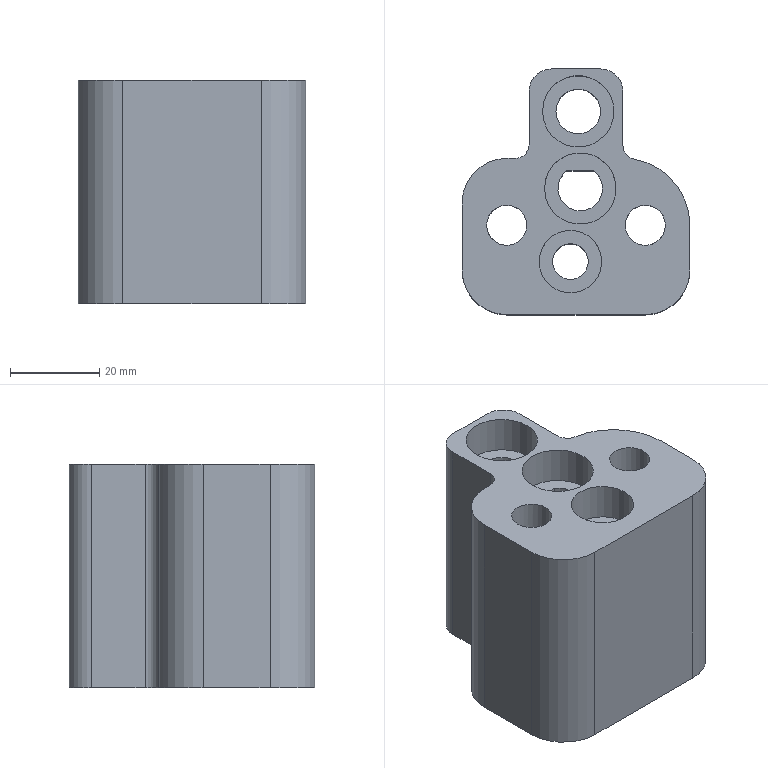Part | STEP file | PN_0021_id1034_x_t | 1 solid | 33 faces | box 51 x 55 x 50 mm | volume 79399 mm3 | cylinder 18 | plane 15 | commonest cylinder face diameters 10 x4 14 x3 20 x3 6 x2 9 x2 16 x2
STEP:
#1=CARTESIAN_POINT('',(276.,-8.,45.));
#2=VERTEX_POINT('',#1);
#3=CARTESIAN_POINT('',(276.,-20.224,45.));
#4=VERTEX_POINT('',#3);
#5=CARTESIAN_POINT('',(276.,-28.807,45.));
#6=DIRECTION('',(0.,-1.,0.));
#7=VECTOR('',#6,1.);
#8=LINE('',#5,#7);
#9=EDGE_CURVE('',#2,#4,#8,.T.);
#10=ORIENTED_EDGE('',*,*,#9,.F.);
#11=CARTESIAN_POINT('',(276.,-8.,95.));
#12=VERTEX_POINT('',#11);
#13=CARTESIAN_POINT('',(276.,-8.,95.));
#14=DIRECTION('',(0.,0.,1.));
#15=VECTOR('',#14,1.);
#16=LINE('',#13,#15);
#17=EDGE_CURVE('',#2,#12,#16,.T.);
#18=ORIENTED_EDGE('',*,*,#17,.T.);
#19=CARTESIAN_POINT('',(276.,-20.224,95.));
#20=VERTEX_POINT('',#19);
#21=CARTESIAN_POINT('',(276.,-28.807,95.));
#22=DIRECTION('',(0.,1.,0.));
#23=VECTOR('',#22,1.);
#24=LINE('',#21,#23);
#25=EDGE_CURVE('',#20,#12,#24,.T.);
#26=ORIENTED_EDGE('',*,*,#25,.F.);
#27=CARTESIAN_POINT('',(276.,-20.224,95.));
#28=DIRECTION('',(0.,0.,1.));
#29=VECTOR('',#28,1.);
#30=LINE('',#27,#29);
#31=EDGE_CURVE('',#4,#20,#30,.T.);
#32=ORIENTED_EDGE('',*,*,#31,.F.);
#33=EDGE_LOOP('',(#10,#18,#26,#32));
#34=FACE_OUTER_BOUND('',#33,.T.);
#35=CARTESIAN_POINT('',(276.,-28.807,95.));
#36=DIRECTION('',(1.,0.,0.));
#37=DIRECTION('',(0.,0.,-1.));
#38=AXIS2_PLACEMENT_3D('',#35,#36,#37);
#39=PLANE('',#38);
#40=ADVANCED_FACE('',(#34),#39,.T.);
#41=CARTESIAN_POINT('',(255.,-8.,95.));
#42=VERTEX_POINT('',#41);
#43=CARTESIAN_POINT('',(255.,-20.,95.));
#44=VERTEX_POINT('',#43);
#45=CARTESIAN_POINT('',(255.,-28.807,95.));
#46=DIRECTION('',(0.,-1.,0.));
#47=VECTOR('',#46,1.);
#48=LINE('',#45,#47);
#49=EDGE_CURVE('',#42,#44,#48,.T.);
#50=ORIENTED_EDGE('',*,*,#49,.F.);
#51=CARTESIAN_POINT('',(255.,-8.,45.));
#52=VERTEX_POINT('',#51);
#53=CARTESIAN_POINT('',(255.,-8.,95.));
#54=DIRECTION('',(0.,0.,-1.));
#55=VECTOR('',#54,1.);
#56=LINE('',#53,#55);
#57=EDGE_CURVE('',#42,#52,#56,.T.);
#58=ORIENTED_EDGE('',*,*,#57,.T.);
#59=CARTESIAN_POINT('',(255.,-20.,45.));
#60=VERTEX_POINT('',#59);
#61=CARTESIAN_POINT('',(255.,-28.807,45.));
#62=DIRECTION('',(0.,1.,0.));
#63=VECTOR('',#62,1.);
#64=LINE('',#61,#63);
#65=EDGE_CURVE('',#60,#52,#64,.T.);
#66=ORIENTED_EDGE('',*,*,#65,.F.);
#67=CARTESIAN_POINT('',(255.,-20.,95.));
#68=DIRECTION('',(0.,0.,-1.));
#69=VECTOR('',#68,1.);
#70=LINE('',#67,#69);
#71=EDGE_CURVE('',#44,#60,#70,.T.);
#72=ORIENTED_EDGE('',*,*,#71,.F.);
#73=EDGE_LOOP('',(#50,#58,#66,#72));
#74=FACE_OUTER_BOUND('',#73,.T.);
#75=CARTESIAN_POINT('',(255.,-28.807,95.));
#76=DIRECTION('',(-1.,0.,0.));
#77=DIRECTION('',(0.,0.,1.));
#78=AXIS2_PLACEMENT_3D('',#75,#76,#77);
#79=PLANE('',#78);
#80=ADVANCED_FACE('',(#74),#79,.T.);
#81=CARTESIAN_POINT('',(271.,-12.5,45.));
#82=VERTEX_POINT('',#81);
#83=CARTESIAN_POINT('',(266.,-12.5,45.));
#84=DIRECTION('',(0.,0.,-1.));
#85=DIRECTION('',(1.,0.,0.));
#86=AXIS2_PLACEMENT_3D('',#83,#84,#85);
#87=CIRCLE('',#86,5.);
#88=EDGE_CURVE('',#82,#82,#87,.T.);
#89=ORIENTED_EDGE('',*,*,#88,.F.);
#90=EDGE_LOOP('',(#89));
#91=FACE_BOUND('',#90,.T.);
#92=CARTESIAN_POINT('',(268.25,-46.114,45.));
#93=VERTEX_POINT('',#92);
#94=CARTESIAN_POINT('',(264.25,-46.114,45.));
#95=DIRECTION('',(0.,0.,-1.));
#96=DIRECTION('',(1.,0.,0.));
#97=AXIS2_PLACEMENT_3D('',#94,#95,#96);
#98=CIRCLE('',#97,4.);
#99=EDGE_CURVE('',#93,#93,#98,.T.);
#100=ORIENTED_EDGE('',*,*,#99,.F.);
#101=EDGE_LOOP('',(#100));
#102=FACE_BOUND('',#101,.T.);
#103=CARTESIAN_POINT('',(263.45,-25.762,45.));
#104=VERTEX_POINT('',#103);
#105=CARTESIAN_POINT('',(269.45,-25.762,45.));
#106=VERTEX_POINT('',#105);
#107=CARTESIAN_POINT('',(266.45,-25.762,45.));
#108=DIRECTION('',(1.,0.,0.));
#109=VECTOR('',#108,1.);
#110=LINE('',#107,#109);
#111=EDGE_CURVE('',#104,#106,#110,.T.);
#112=ORIENTED_EDGE('',*,*,#111,.F.);
#113=CARTESIAN_POINT('',(266.45,-29.762,45.));
#114=DIRECTION('',(0.,0.,-1.));
#115=DIRECTION('',(1.,0.,0.));
#116=AXIS2_PLACEMENT_3D('',#113,#114,#115);
#117=CIRCLE('',#116,5.);
#118=EDGE_CURVE('',#106,#104,#117,.T.);
#119=ORIENTED_EDGE('',*,*,#118,.F.);
#120=EDGE_LOOP('',(#112,#119));
#121=FACE_BOUND('',#120,.T.);
#122=CARTESIAN_POINT('',(250.,-31.,45.));
#123=VERTEX_POINT('',#122);
#124=CARTESIAN_POINT('',(250.,-38.,45.));
#125=DIRECTION('',(0.,0.,-1.));
#126=DIRECTION('',(0.,1.,0.));
#127=AXIS2_PLACEMENT_3D('',#124,#125,#126);
#128=CIRCLE('',#127,7.);
#129=EDGE_CURVE('',#123,#123,#128,.T.);
#130=ORIENTED_EDGE('',*,*,#129,.F.);
#131=EDGE_LOOP('',(#130));
#132=FACE_BOUND('',#131,.T.);
#133=CARTESIAN_POINT('',(281.,-45.,45.));
#134=VERTEX_POINT('',#133);
#135=CARTESIAN_POINT('',(281.,-38.,45.));
#136=DIRECTION('',(0.,0.,-1.));
#137=DIRECTION('',(0.,-1.,0.));
#138=AXIS2_PLACEMENT_3D('',#135,#136,#137);
#139=CIRCLE('',#138,7.);
#140=EDGE_CURVE('',#134,#134,#139,.T.);
#141=ORIENTED_EDGE('',*,*,#140,.F.);
#142=EDGE_LOOP('',(#141));
#143=FACE_BOUND('',#142,.T.);
#144=CARTESIAN_POINT('',(278.5,-23.182,45.));
#145=VERTEX_POINT('',#144);
#146=CARTESIAN_POINT('',(279.,-20.224,45.));
#147=DIRECTION('',(0.,0.,-1.));
#148=DIRECTION('',(1.,0.,0.));
#149=AXIS2_PLACEMENT_3D('',#146,#147,#148);
#150=CIRCLE('',#149,3.);
#151=EDGE_CURVE('',#145,#4,#150,.T.);
#152=ORIENTED_EDGE('',*,*,#151,.F.);
#153=CARTESIAN_POINT('',(291.,-37.972,45.));
#154=VERTEX_POINT('',#153);
#155=CARTESIAN_POINT('',(276.,-37.972,45.));
#156=DIRECTION('',(0.,0.,-1.));
#157=DIRECTION('',(1.,0.,0.));
#158=AXIS2_PLACEMENT_3D('',#155,#156,#157);
#159=CIRCLE('',#158,15.);
#160=EDGE_CURVE('',#145,#154,#159,.T.);
#161=ORIENTED_EDGE('',*,*,#160,.T.);
#162=CARTESIAN_POINT('',(291.,-48.,45.));
#163=VERTEX_POINT('',#162);
#164=CARTESIAN_POINT('',(291.,-28.807,45.));
#165=DIRECTION('',(0.,1.,0.));
#166=VECTOR('',#165,1.);
#167=LINE('',#164,#166);
#168=EDGE_CURVE('',#163,#154,#167,.T.);
#169=ORIENTED_EDGE('',*,*,#168,.F.);
#170=CARTESIAN_POINT('',(281.,-58.,45.));
#171=VERTEX_POINT('',#170);
#172=CARTESIAN_POINT('',(281.,-48.,45.));
#173=DIRECTION('',(0.,0.,-1.));
#174=DIRECTION('',(1.,0.,0.));
#175=AXIS2_PLACEMENT_3D('',#172,#173,#174);
#176=CIRCLE('',#175,10.);
#177=EDGE_CURVE('',#163,#171,#176,.T.);
#178=ORIENTED_EDGE('',*,*,#177,.T.);
#179=CARTESIAN_POINT('',(250.,-58.,45.));
#180=VERTEX_POINT('',#179);
#181=CARTESIAN_POINT('',(265.85,-58.,45.));
#182=DIRECTION('',(-1.,0.,0.));
#183=VECTOR('',#182,1.);
#184=LINE('',#181,#183);
#185=EDGE_CURVE('',#171,#180,#184,.T.);
#186=ORIENTED_EDGE('',*,*,#185,.T.);
#187=CARTESIAN_POINT('',(240.,-48.,45.));
#188=VERTEX_POINT('',#187);
#189=CARTESIAN_POINT('',(250.,-48.,45.));
#190=DIRECTION('',(0.,0.,-1.));
#191=DIRECTION('',(1.,0.,0.));
#192=AXIS2_PLACEMENT_3D('',#189,#190,#191);
#193=CIRCLE('',#192,10.);
#194=EDGE_CURVE('',#180,#188,#193,.T.);
#195=ORIENTED_EDGE('',*,*,#194,.T.);
#196=CARTESIAN_POINT('',(240.,-33.,45.));
#197=VERTEX_POINT('',#196);
#198=CARTESIAN_POINT('',(240.,-58.,45.));
#199=DIRECTION('',(0.,1.,0.));
#200=VECTOR('',#199,1.);
#201=LINE('',#198,#200);
#202=EDGE_CURVE('',#188,#197,#201,.T.);
#203=ORIENTED_EDGE('',*,*,#202,.T.);
#204=CARTESIAN_POINT('',(250.,-23.,45.));
#205=VERTEX_POINT('',#204);
#206=CARTESIAN_POINT('',(250.,-33.,45.));
#207=DIRECTION('',(0.,0.,-1.));
#208=DIRECTION('',(1.,0.,0.));
#209=AXIS2_PLACEMENT_3D('',#206,#207,#208);
#210=CIRCLE('',#209,10.);
#211=EDGE_CURVE('',#197,#205,#210,.T.);
#212=ORIENTED_EDGE('',*,*,#211,.T.);
#213=CARTESIAN_POINT('',(252.,-23.,45.));
#214=VERTEX_POINT('',#213);
#215=CARTESIAN_POINT('',(267.85,-23.,45.));
#216=DIRECTION('',(-1.,0.,0.));
#217=VECTOR('',#216,1.);
#218=LINE('',#215,#217);
#219=EDGE_CURVE('',#214,#205,#218,.T.);
#220=ORIENTED_EDGE('',*,*,#219,.F.);
#221=CARTESIAN_POINT('',(252.,-20.,45.));
#222=DIRECTION('',(0.,0.,-1.));
#223=DIRECTION('',(1.,0.,0.));
#224=AXIS2_PLACEMENT_3D('',#221,#222,#223);
#225=CIRCLE('',#224,3.);
#226=EDGE_CURVE('',#60,#214,#225,.T.);
#227=ORIENTED_EDGE('',*,*,#226,.F.);
#228=ORIENTED_EDGE('',*,*,#65,.T.);
#229=CARTESIAN_POINT('',(260.,-3.,45.));
#230=VERTEX_POINT('',#229);
#231=CARTESIAN_POINT('',(260.,-8.,45.));
#232=DIRECTION('',(0.,0.,-1.));
#233=DIRECTION('',(1.,0.,0.));
#234=AXIS2_PLACEMENT_3D('',#231,#232,#233);
#235=CIRCLE('',#234,5.);
#236=EDGE_CURVE('',#52,#230,#235,.T.);
#237=ORIENTED_EDGE('',*,*,#236,.T.);
#238=CARTESIAN_POINT('',(271.,-3.,45.));
#239=VERTEX_POINT('',#238);
#240=CARTESIAN_POINT('',(265.85,-3.,45.));
#241=DIRECTION('',(1.,0.,0.));
#242=VECTOR('',#241,1.);
#243=LINE('',#240,#242);
#244=EDGE_CURVE('',#230,#239,#243,.T.);
#245=ORIENTED_EDGE('',*,*,#244,.T.);
#246=CARTESIAN_POINT('',(271.,-8.,45.));
#247=DIRECTION('',(0.,0.,-1.));
#248=DIRECTION('',(1.,0.,0.));
#249=AXIS2_PLACEMENT_3D('',#246,#247,#248);
#250=CIRCLE('',#249,5.);
#251=EDGE_CURVE('',#239,#2,#250,.T.);
#252=ORIENTED_EDGE('',*,*,#251,.T.);
#253=ORIENTED_EDGE('',*,*,#9,.T.);
#254=EDGE_LOOP('',(#152,#161,#169,#178,#186,#195,#203,#212,#220,#227,#228,#237,#245,#252,#253));
#255=FACE_BOUND('',#254,.T.);
#256=CARTESIAN_POINT('',(265.85,-28.807,45.));
#257=DIRECTION('',(0.,0.,1.));
#258=DIRECTION('',(1.,0.,0.));
#259=AXIS2_PLACEMENT_3D('',#256,#257,#258);
#260=PLANE('',#259);
#261=ADVANCED_FACE('',(#91,#102,#121,#132,#143,#255),#260,.F.);
#262=ORIENTED_EDGE('',*,*,#244,.F.);
#263=CARTESIAN_POINT('',(260.,-3.,95.));
#264=VERTEX_POINT('',#263);
#265=CARTESIAN_POINT('',(260.,-3.,95.));
#266=DIRECTION('',(0.,0.,1.));
#267=VECTOR('',#266,1.);
#268=LINE('',#265,#267);
#269=EDGE_CURVE('',#230,#264,#268,.T.);
#270=ORIENTED_EDGE('',*,*,#269,.T.);
#271=CARTESIAN_POINT('',(271.,-3.,95.));
#272=VERTEX_POINT('',#271);
#273=CARTESIAN_POINT('',(265.85,-3.,95.));
#274=DIRECTION('',(-1.,0.,0.));
#275=VECTOR('',#274,1.);
#276=LINE('',#273,#275);
#277=EDGE_CURVE('',#272,#264,#276,.T.);
#278=ORIENTED_EDGE('',*,*,#277,.F.);
#279=CARTESIAN_POINT('',(271.,-3.,95.));
#280=DIRECTION('',(0.,0.,-1.));
#281=VECTOR('',#280,1.);
#282=LINE('',#279,#281);
#283=EDGE_CURVE('',#272,#239,#282,.T.);
#284=ORIENTED_EDGE('',*,*,#283,.T.);
#285=EDGE_LOOP('',(#262,#270,#278,#284));
#286=FACE_OUTER_BOUND('',#285,.T.);
#287=CARTESIAN_POINT('',(265.85,-3.,95.));
#288=DIRECTION('',(0.,1.,0.));
#289=DIRECTION('',(0.,0.,-1.));
#290=AXIS2_PLACEMENT_3D('',#287,#288,#289);
#291=PLANE('',#290);
#292=ADVANCED_FACE('',(#286),#291,.T.);
#293=ORIENTED_EDGE('',*,*,#185,.F.);
#294=CARTESIAN_POINT('',(281.,-58.,95.));
#295=VERTEX_POINT('',#294);
#296=CARTESIAN_POINT('',(281.,-58.,95.));
#297=DIRECTION('',(0.,0.,1.));
#298=VECTOR('',#297,1.);
#299=LINE('',#296,#298);
#300=EDGE_CURVE('',#171,#295,#299,.T.);
#301=ORIENTED_EDGE('',*,*,#300,.T.);
#302=CARTESIAN_POINT('',(250.,-58.,95.));
#303=VERTEX_POINT('',#302);
#304=CARTESIAN_POINT('',(265.85,-58.,95.));
#305=DIRECTION('',(1.,0.,0.));
#306=VECTOR('',#305,1.);
#307=LINE('',#304,#306);
#308=EDGE_CURVE('',#303,#295,#307,.T.);
#309=ORIENTED_EDGE('',*,*,#308,.F.);
#310=CARTESIAN_POINT('',(250.,-58.,45.));
#311=DIRECTION('',(0.,0.,-1.));
#312=VECTOR('',#311,1.);
#313=LINE('',#310,#312);
#314=EDGE_CURVE('',#303,#180,#313,.T.);
#315=ORIENTED_EDGE('',*,*,#314,.T.);
#316=EDGE_LOOP('',(#293,#301,#309,#315));
#317=FACE_OUTER_BOUND('',#316,.T.);
#318=CARTESIAN_POINT('',(265.85,-58.,95.));
#319=DIRECTION('',(0.,-1.,0.));
#320=DIRECTION('',(0.,0.,1.));
#321=AXIS2_PLACEMENT_3D('',#318,#319,#320);
#322=PLANE('',#321);
#323=ADVANCED_FACE('',(#317),#322,.T.);
#324=CARTESIAN_POINT('',(274.,-12.5,95.));
#325=VERTEX_POINT('',#324);
#326=CARTESIAN_POINT('',(266.,-12.5,95.));
#327=DIRECTION('',(0.,0.,1.));
#328=DIRECTION('',(1.,0.,0.));
#329=AXIS2_PLACEMENT_3D('',#326,#327,#328);
#330=CIRCLE('',#329,8.);
#331=EDGE_CURVE('',#325,#325,#330,.T.);
#332=ORIENTED_EDGE('',*,*,#331,.F.);
#333=EDGE_LOOP('',(#332));
#334=FACE_BOUND('',#333,.T.);
#335=CARTESIAN_POINT('',(271.25,-46.114,95.));
#336=VERTEX_POINT('',#335);
#337=CARTESIAN_POINT('',(264.25,-46.114,95.));
#338=DIRECTION('',(0.,0.,1.));
#339=DIRECTION('',(1.,0.,0.));
#340=AXIS2_PLACEMENT_3D('',#337,#338,#339);
#341=CIRCLE('',#340,7.);
#342=EDGE_CURVE('',#336,#336,#341,.T.);
#343=ORIENTED_EDGE('',*,*,#342,.F.);
#344=EDGE_LOOP('',(#343));
#345=FACE_BOUND('',#344,.T.);
#346=CARTESIAN_POINT('',(274.45,-29.762,95.));
#347=VERTEX_POINT('',#346);
#348=CARTESIAN_POINT('',(266.45,-29.762,95.));
#349=DIRECTION('',(0.,0.,1.));
#350=DIRECTION('',(1.,0.,0.));
#351=AXIS2_PLACEMENT_3D('',#348,#349,#350);
#352=CIRCLE('',#351,8.);
#353=EDGE_CURVE('',#347,#347,#352,.T.);
#354=ORIENTED_EDGE('',*,*,#353,.F.);
#355=EDGE_LOOP('',(#354));
#356=FACE_BOUND('',#355,.T.);
#357=CARTESIAN_POINT('',(254.5,-38.,95.));
#358=VERTEX_POINT('',#357);
#359=CARTESIAN_POINT('',(250.,-38.,95.));
#360=DIRECTION('',(0.,0.,1.));
#361=DIRECTION('',(1.,0.,0.));
#362=AXIS2_PLACEMENT_3D('',#359,#360,#361);
#363=CIRCLE('',#362,4.5);
#364=EDGE_CURVE('',#358,#358,#363,.T.);
#365=ORIENTED_EDGE('',*,*,#364,.F.);
#366=EDGE_LOOP('',(#365));
#367=FACE_BOUND('',#366,.T.);
#368=CARTESIAN_POINT('',(285.5,-38.,95.));
#369=VERTEX_POINT('',#368);
#370=CARTESIAN_POINT('',(281.,-38.,95.));
#371=DIRECTION('',(0.,0.,1.));
#372=DIRECTION('',(1.,0.,0.));
#373=AXIS2_PLACEMENT_3D('',#370,#371,#372);
#374=CIRCLE('',#373,4.5);
#375=EDGE_CURVE('',#369,#369,#374,.T.);
#376=ORIENTED_EDGE('',*,*,#375,.F.);
#377=EDGE_LOOP('',(#376));
#378=FACE_BOUND('',#377,.T.);
#379=CARTESIAN_POINT('',(291.,-48.,95.));
#380=VERTEX_POINT('',#379);
#381=CARTESIAN_POINT('',(291.,-37.972,95.));
#382=VERTEX_POINT('',#381);
#383=CARTESIAN_POINT('',(291.,-58.,95.));
#384=DIRECTION('',(0.,1.,0.));
#385=VECTOR('',#384,1.);
#386=LINE('',#383,#385);
#387=EDGE_CURVE('',#380,#382,#386,.T.);
#388=ORIENTED_EDGE('',*,*,#387,.T.);
#389=CARTESIAN_POINT('',(278.5,-23.182,95.));
#390=VERTEX_POINT('',#389);
#391=CARTESIAN_POINT('',(276.,-37.972,95.));
#392=DIRECTION('',(0.,0.,1.));
#393=DIRECTION('',(1.,0.,0.));
#394=AXIS2_PLACEMENT_3D('',#391,#392,#393);
#395=CIRCLE('',#394,15.);
#396=EDGE_CURVE('',#382,#390,#395,.T.);
#397=ORIENTED_EDGE('',*,*,#396,.T.);
#398=CARTESIAN_POINT('',(279.,-20.224,95.));
#399=DIRECTION('',(0.,0.,1.));
#400=DIRECTION('',(1.,0.,0.));
#401=AXIS2_PLACEMENT_3D('',#398,#399,#400);
#402=CIRCLE('',#401,3.);
#403=EDGE_CURVE('',#20,#390,#402,.T.);
#404=ORIENTED_EDGE('',*,*,#403,.F.);
#405=ORIENTED_EDGE('',*,*,#25,.T.);
#406=CARTESIAN_POINT('',(271.,-8.,95.));
#407=DIRECTION('',(0.,0.,1.));
#408=DIRECTION('',(1.,0.,0.));
#409=AXIS2_PLACEMENT_3D('',#406,#407,#408);
#410=CIRCLE('',#409,5.);
#411=EDGE_CURVE('',#12,#272,#410,.T.);
#412=ORIENTED_EDGE('',*,*,#411,.T.);
#413=ORIENTED_EDGE('',*,*,#277,.T.);
#414=CARTESIAN_POINT('',(260.,-8.,95.));
#415=DIRECTION('',(0.,0.,1.));
#416=DIRECTION('',(1.,0.,0.));
#417=AXIS2_PLACEMENT_3D('',#414,#415,#416);
#418=CIRCLE('',#417,5.);
#419=EDGE_CURVE('',#264,#42,#418,.T.);
#420=ORIENTED_EDGE('',*,*,#419,.T.);
#421=ORIENTED_EDGE('',*,*,#49,.T.);
#422=CARTESIAN_POINT('',(252.,-23.,95.));
#423=VERTEX_POINT('',#422);
#424=CARTESIAN_POINT('',(252.,-20.,95.));
#425=DIRECTION('',(0.,0.,1.));
#426=DIRECTION('',(1.,0.,0.));
#427=AXIS2_PLACEMENT_3D('',#424,#425,#426);
#428=CIRCLE('',#427,3.);
#429=EDGE_CURVE('',#423,#44,#428,.T.);
#430=ORIENTED_EDGE('',*,*,#429,.F.);
#431=CARTESIAN_POINT('',(250.,-23.,95.));
#432=VERTEX_POINT('',#431);
#433=CARTESIAN_POINT('',(267.85,-23.,95.));
#434=DIRECTION('',(1.,0.,0.));
#435=VECTOR('',#434,1.);
#436=LINE('',#433,#435);
#437=EDGE_CURVE('',#432,#423,#436,.T.);
#438=ORIENTED_EDGE('',*,*,#437,.F.);
#439=CARTESIAN_POINT('',(240.,-33.,95.));
#440=VERTEX_POINT('',#439);
#441=CARTESIAN_POINT('',(250.,-33.,95.));
#442=DIRECTION('',(0.,0.,1.));
#443=DIRECTION('',(1.,0.,0.));
#444=AXIS2_PLACEMENT_3D('',#441,#442,#443);
#445=CIRCLE('',#444,10.);
#446=EDGE_CURVE('',#432,#440,#445,.T.);
#447=ORIENTED_EDGE('',*,*,#446,.T.);
#448=CARTESIAN_POINT('',(240.,-48.,95.));
#449=VERTEX_POINT('',#448);
#450=CARTESIAN_POINT('',(240.,-28.807,95.));
#451=DIRECTION('',(0.,1.,0.));
#452=VECTOR('',#451,1.);
#453=LINE('',#450,#452);
#454=EDGE_CURVE('',#449,#440,#453,.T.);
#455=ORIENTED_EDGE('',*,*,#454,.F.);
#456=CARTESIAN_POINT('',(250.,-48.,95.));
#457=DIRECTION('',(0.,0.,1.));
#458=DIRECTION('',(1.,0.,0.));
#459=AXIS2_PLACEMENT_3D('',#456,#457,#458);
#460=CIRCLE('',#459,10.);
#461=EDGE_CURVE('',#449,#303,#460,.T.);
#462=ORIENTED_EDGE('',*,*,#461,.T.);
#463=ORIENTED_EDGE('',*,*,#308,.T.);
#464=CARTESIAN_POINT('',(281.,-48.,95.));
#465=DIRECTION('',(0.,0.,1.));
#466=DIRECTION('',(1.,0.,0.));
#467=AXIS2_PLACEMENT_3D('',#464,#465,#466);
#468=CIRCLE('',#467,10.);
#469=EDGE_CURVE('',#295,#380,#468,.T.);
#470=ORIENTED_EDGE('',*,*,#469,.T.);
#471=EDGE_LOOP('',(#388,#397,#404,#405,#412,#413,#420,#421,#430,#438,#447,#455,#462,#463,#470));
#472=FACE_BOUND('',#471,.T.);
#473=CARTESIAN_POINT('',(265.85,-28.807,95.));
#474=DIRECTION('',(0.,0.,1.));
#475=DIRECTION('',(1.,0.,0.));
#476=AXIS2_PLACEMENT_3D('',#473,#474,#475);
#477=PLANE('',#476);
#478=ADVANCED_FACE('',(#334,#345,#356,#367,#378,#472),#477,.T.);
#479=ORIENTED_EDGE('',*,*,#454,.T.);
#480=CARTESIAN_POINT('',(240.,-33.,95.));
#481=DIRECTION('',(0.,0.,-1.));
#482=VECTOR('',#481,1.);
#483=LINE('',#480,#482);
#484=EDGE_CURVE('',#440,#197,#483,.T.);
#485=ORIENTED_EDGE('',*,*,#484,.T.);
#486=ORIENTED_EDGE('',*,*,#202,.F.);
#487=CARTESIAN_POINT('',(240.,-48.,95.));
#488=DIRECTION('',(0.,0.,1.));
#489=VECTOR('',#488,1.);
#490=LINE('',#487,#489);
#491=EDGE_CURVE('',#188,#449,#490,.T.);
#492=ORIENTED_EDGE('',*,*,#491,.T.);
#493=EDGE_LOOP('',(#479,#485,#486,#492));
#494=FACE_OUTER_BOUND('',#493,.T.);
#495=CARTESIAN_POINT('',(240.,-58.,95.));
#496=DIRECTION('',(1.,0.,0.));
#497=DIRECTION('',(0.,0.,-1.));
#498=AXIS2_PLACEMENT_3D('',#495,#496,#497);
#499=PLANE('',#498);
#500=ADVANCED_FACE('',(#494),#499,.F.);
#501=ORIENTED_EDGE('',*,*,#219,.T.);
#502=CARTESIAN_POINT('',(250.,-23.,95.));
#503=DIRECTION('',(0.,0.,1.));
#504=VECTOR('',#503,1.);
#505=LINE('',#502,#504);
#506=EDGE_CURVE('',#205,#432,#505,.T.);
#507=ORIENTED_EDGE('',*,*,#506,.T.);
#508=ORIENTED_EDGE('',*,*,#437,.T.);
#509=CARTESIAN_POINT('',(252.,-23.,95.));
#510=DIRECTION('',(0.,0.,1.));
#511=VECTOR('',#510,1.);
#512=LINE('',#509,#511);
#513=EDGE_CURVE('',#214,#423,#512,.T.);
#514=ORIENTED_EDGE('',*,*,#513,.F.);
#515=EDGE_LOOP('',(#501,#507,#508,#514));
#516=FACE_OUTER_BOUND('',#515,.T.);
#517=CARTESIAN_POINT('',(267.85,-23.,95.));
#518=DIRECTION('',(0.,-1.,0.));
#519=DIRECTION('',(0.,0.,1.));
#520=AXIS2_PLACEMENT_3D('',#517,#518,#519);
#521=PLANE('',#520);
#522=ADVANCED_FACE('',(#516),#521,.F.);
#523=ORIENTED_EDGE('',*,*,#168,.T.);
#524=CARTESIAN_POINT('',(291.,-37.972,95.));
#525=DIRECTION('',(0.,0.,1.));
#526=VECTOR('',#525,1.);
#527=LINE('',#524,#526);
#528=EDGE_CURVE('',#154,#382,#527,.T.);
#529=ORIENTED_EDGE('',*,*,#528,.T.);
#530=ORIENTED_EDGE('',*,*,#387,.F.);
#531=CARTESIAN_POINT('',(291.,-48.,45.));
#532=DIRECTION('',(0.,0.,-1.));
#533=VECTOR('',#532,1.);
#534=LINE('',#531,#533);
#535=EDGE_CURVE('',#380,#163,#534,.T.);
#536=ORIENTED_EDGE('',*,*,#535,.T.);
#537=EDGE_LOOP('',(#523,#529,#530,#536));
#538=FACE_OUTER_BOUND('',#537,.T.);
#539=CARTESIAN_POINT('',(291.,-58.,95.));
#540=DIRECTION('',(1.,0.,0.));
#541=DIRECTION('',(0.,0.,-1.));
#542=AXIS2_PLACEMENT_3D('',#539,#540,#541);
#543=PLANE('',#542);
#544=ADVANCED_FACE('',(#538),#543,.T.);
#545=ORIENTED_EDGE('',*,*,#403,.T.);
#546=CARTESIAN_POINT('',(278.5,-23.182,95.));
#547=DIRECTION('',(0.,0.,-1.));
#548=VECTOR('',#547,1.);
#549=LINE('',#546,#548);
#550=EDGE_CURVE('',#390,#145,#549,.T.);
#551=ORIENTED_EDGE('',*,*,#550,.T.);
#552=ORIENTED_EDGE('',*,*,#151,.T.);
#553=ORIENTED_EDGE('',*,*,#31,.T.);
#554=EDGE_LOOP('',(#545,#551,#552,#553));
#555=FACE_OUTER_BOUND('',#554,.T.);
#556=CARTESIAN_POINT('',(279.,-20.224,95.));
#557=DIRECTION('',(0.,0.,1.));
#558=DIRECTION('',(1.,0.,0.));
#559=AXIS2_PLACEMENT_3D('',#556,#557,#558);
#560=CYLINDRICAL_SURFACE('',#559,3.);
#561=ADVANCED_FACE('',(#555),#560,.F.);
#562=ORIENTED_EDGE('',*,*,#429,.T.);
#563=ORIENTED_EDGE('',*,*,#71,.T.);
#564=ORIENTED_EDGE('',*,*,#226,.T.);
#565=ORIENTED_EDGE('',*,*,#513,.T.);
#566=EDGE_LOOP('',(#562,#563,#564,#565));
#567=FACE_OUTER_BOUND('',#566,.T.);
#568=CARTESIAN_POINT('',(252.,-20.,95.));
#569=DIRECTION('',(0.,0.,-1.));
#570=DIRECTION('',(-1.,0.,0.));
#571=AXIS2_PLACEMENT_3D('',#568,#569,#570);
#572=CYLINDRICAL_SURFACE('',#571,3.);
#573=ADVANCED_FACE('',(#567),#572,.F.);
#574=ORIENTED_EDGE('',*,*,#446,.F.);
#575=ORIENTED_EDGE('',*,*,#506,.F.);
#576=ORIENTED_EDGE('',*,*,#211,.F.);
#577=ORIENTED_EDGE('',*,*,#484,.F.);
#578=EDGE_LOOP('',(#574,#575,#576,#577));
#579=FACE_OUTER_BOUND('',#578,.T.);
#580=CARTESIAN_POINT('',(250.,-33.,95.));
#581=DIRECTION('',(0.,0.,-1.));
#582=DIRECTION('',(-1.,0.,0.));
#583=AXIS2_PLACEMENT_3D('',#580,#581,#582);
#584=CYLINDRICAL_SURFACE('',#583,10.);
#585=ADVANCED_FACE('',(#579),#584,.T.);
#586=ORIENTED_EDGE('',*,*,#469,.F.);
#587=ORIENTED_EDGE('',*,*,#300,.F.);
#588=ORIENTED_EDGE('',*,*,#177,.F.);
#589=ORIENTED_EDGE('',*,*,#535,.F.);
#590=EDGE_LOOP('',(#586,#587,#588,#589));
#591=FACE_OUTER_BOUND('',#590,.T.);
#592=CARTESIAN_POINT('',(281.,-48.,95.));
#593=DIRECTION('',(0.,0.,-1.));
#594=DIRECTION('',(-1.,0.,0.));
#595=AXIS2_PLACEMENT_3D('',#592,#593,#594);
#596=CYLINDRICAL_SURFACE('',#595,10.);
#597=ADVANCED_FACE('',(#591),#596,.T.);
#598=ORIENTED_EDGE('',*,*,#461,.F.);
#599=ORIENTED_EDGE('',*,*,#491,.F.);
#600=ORIENTED_EDGE('',*,*,#194,.F.);
#601=ORIENTED_EDGE('',*,*,#314,.F.);
#602=EDGE_LOOP('',(#598,#599,#600,#601));
#603=FACE_OUTER_BOUND('',#602,.T.);
#604=CARTESIAN_POINT('',(250.,-48.,95.));
#605=DIRECTION('',(0.,0.,1.));
#606=DIRECTION('',(1.,0.,0.));
#607=AXIS2_PLACEMENT_3D('',#604,#605,#606);
#608=CYLINDRICAL_SURFACE('',#607,10.);
#609=ADVANCED_FACE('',(#603),#608,.T.);
#610=ORIENTED_EDGE('',*,*,#419,.F.);
#611=ORIENTED_EDGE('',*,*,#269,.F.);
#612=ORIENTED_EDGE('',*,*,#236,.F.);
#613=ORIENTED_EDGE('',*,*,#57,.F.);
#614=EDGE_LOOP('',(#610,#611,#612,#613));
#615=FACE_OUTER_BOUND('',#614,.T.);
#616=CARTESIAN_POINT('',(260.,-8.,95.));
#617=DIRECTION('',(0.,0.,-1.));
#618=DIRECTION('',(-1.,0.,0.));
#619=AXIS2_PLACEMENT_3D('',#616,#617,#618);
#620=CYLINDRICAL_SURFACE('',#619,5.);
#621=ADVANCED_FACE('',(#615),#620,.T.);
#622=ORIENTED_EDGE('',*,*,#411,.F.);
#623=ORIENTED_EDGE('',*,*,#17,.F.);
#624=ORIENTED_EDGE('',*,*,#251,.F.);
#625=ORIENTED_EDGE('',*,*,#283,.F.);
#626=EDGE_LOOP('',(#622,#623,#624,#625));
#627=FACE_OUTER_BOUND('',#626,.T.);
#628=CARTESIAN_POINT('',(271.,-8.,95.));
#629=DIRECTION('',(0.,0.,-1.));
#630=DIRECTION('',(-1.,0.,0.));
#631=AXIS2_PLACEMENT_3D('',#628,#629,#630);
#632=CYLINDRICAL_SURFACE('',#631,5.);
#633=ADVANCED_FACE('',(#627),#632,.T.);
#634=ORIENTED_EDGE('',*,*,#396,.F.);
#635=ORIENTED_EDGE('',*,*,#528,.F.);
#636=ORIENTED_EDGE('',*,*,#160,.F.);
#637=ORIENTED_EDGE('',*,*,#550,.F.);
#638=EDGE_LOOP('',(#634,#635,#636,#637));
#639=FACE_OUTER_BOUND('',#638,.T.);
#640=CARTESIAN_POINT('',(276.,-37.972,95.));
#641=DIRECTION('',(0.,0.,1.));
#642=DIRECTION('',(1.,0.,0.));
#643=AXIS2_PLACEMENT_3D('',#640,#641,#642);
#644=CYLINDRICAL_SURFACE('',#643,15.);
#645=ADVANCED_FACE('',(#639),#644,.T.);
#646=ORIENTED_EDGE('',*,*,#375,.T.);
#647=EDGE_LOOP('',(#646));
#648=FACE_BOUND('',#647,.T.);
#649=CARTESIAN_POINT('',(281.,-42.5,75.));
#650=VERTEX_POINT('',#649);
#651=CARTESIAN_POINT('',(281.,-38.,75.));
#652=DIRECTION('',(0.,0.,-1.));
#653=DIRECTION('',(0.,-1.,0.));
#654=AXIS2_PLACEMENT_3D('',#651,#652,#653);
#655=CIRCLE('',#654,4.5);
#656=EDGE_CURVE('',#650,#650,#655,.T.);
#657=ORIENTED_EDGE('',*,*,#656,.T.);
#658=EDGE_LOOP('',(#657));
#659=FACE_BOUND('',#658,.T.);
#660=CARTESIAN_POINT('',(281.,-38.,105.));
#661=DIRECTION('',(0.,0.,-1.));
#662=DIRECTION('',(0.,1.,0.));
#663=AXIS2_PLACEMENT_3D('',#660,#661,#662);
#664=CYLINDRICAL_SURFACE('',#663,4.5);
#665=ADVANCED_FACE('',(#648,#659),#664,.F.);
#666=ORIENTED_EDGE('',*,*,#656,.F.);
#667=EDGE_LOOP('',(#666));
#668=FACE_BOUND('',#667,.T.);
#669=CARTESIAN_POINT('',(281.,-31.,75.));
#670=VERTEX_POINT('',#669);
#671=CARTESIAN_POINT('',(281.,-38.,75.));
#672=DIRECTION('',(0.,0.,-1.));
#673=DIRECTION('',(0.,1.,0.));
#674=AXIS2_PLACEMENT_3D('',#671,#672,#673);
#675=CIRCLE('',#674,7.);
#676=EDGE_CURVE('',#670,#670,#675,.T.);
#677=ORIENTED_EDGE('',*,*,#676,.T.);
#678=EDGE_LOOP('',(#677));
#679=FACE_BOUND('',#678,.T.);
#680=CARTESIAN_POINT('',(281.,-38.,75.));
#681=DIRECTION('',(0.,0.,1.));
#682=DIRECTION('',(0.,-1.,0.));
#683=AXIS2_PLACEMENT_3D('',#680,#681,#682);
#684=PLANE('',#683);
#685=ADVANCED_FACE('',(#668,#679),#684,.F.);
#686=ORIENTED_EDGE('',*,*,#140,.T.);
#687=EDGE_LOOP('',(#686));
#688=FACE_BOUND('',#687,.T.);
#689=ORIENTED_EDGE('',*,*,#676,.F.);
#690=EDGE_LOOP('',(#689));
#691=FACE_BOUND('',#690,.T.);
#692=CARTESIAN_POINT('',(281.,-38.,75.));
#693=DIRECTION('',(0.,0.,-1.));
#694=DIRECTION('',(0.,1.,0.));
#695=AXIS2_PLACEMENT_3D('',#692,#693,#694);
#696=CYLINDRICAL_SURFACE('',#695,7.);
#697=ADVANCED_FACE('',(#688,#691),#696,.F.);
#698=ORIENTED_EDGE('',*,*,#364,.T.);
#699=EDGE_LOOP('',(#698));
#700=FACE_BOUND('',#699,.T.);
#701=CARTESIAN_POINT('',(250.,-33.5,75.));
#702=VERTEX_POINT('',#701);
#703=CARTESIAN_POINT('',(250.,-38.,75.));
#704=DIRECTION('',(0.,0.,-1.));
#705=DIRECTION('',(0.,1.,0.));
#706=AXIS2_PLACEMENT_3D('',#703,#704,#705);
#707=CIRCLE('',#706,4.5);
#708=EDGE_CURVE('',#702,#702,#707,.T.);
#709=ORIENTED_EDGE('',*,*,#708,.T.);
#710=EDGE_LOOP('',(#709));
#711=FACE_BOUND('',#710,.T.);
#712=CARTESIAN_POINT('',(250.,-38.,105.));
#713=DIRECTION('',(0.,0.,-1.));
#714=DIRECTION('',(0.,-1.,0.));
#715=AXIS2_PLACEMENT_3D('',#712,#713,#714);
#716=CYLINDRICAL_SURFACE('',#715,4.5);
#717=ADVANCED_FACE('',(#700,#711),#716,.F.);
#718=ORIENTED_EDGE('',*,*,#708,.F.);
#719=EDGE_LOOP('',(#718));
#720=FACE_BOUND('',#719,.T.);
#721=CARTESIAN_POINT('',(250.,-45.,75.));
#722=VERTEX_POINT('',#721);
#723=CARTESIAN_POINT('',(250.,-38.,75.));
#724=DIRECTION('',(0.,0.,-1.));
#725=DIRECTION('',(0.,-1.,0.));
#726=AXIS2_PLACEMENT_3D('',#723,#724,#725);
#727=CIRCLE('',#726,7.);
#728=EDGE_CURVE('',#722,#722,#727,.T.);
#729=ORIENTED_EDGE('',*,*,#728,.T.);
#730=EDGE_LOOP('',(#729));
#731=FACE_BOUND('',#730,.T.);
#732=CARTESIAN_POINT('',(250.,-38.,75.));
#733=DIRECTION('',(0.,0.,1.));
#734=DIRECTION('',(0.,1.,0.));
#735=AXIS2_PLACEMENT_3D('',#732,#733,#734);
#736=PLANE('',#735);
#737=ADVANCED_FACE('',(#720,#731),#736,.F.);
#738=ORIENTED_EDGE('',*,*,#129,.T.);
#739=EDGE_LOOP('',(#738));
#740=FACE_BOUND('',#739,.T.);
#741=ORIENTED_EDGE('',*,*,#728,.F.);
#742=EDGE_LOOP('',(#741));
#743=FACE_BOUND('',#742,.T.);
#744=CARTESIAN_POINT('',(250.,-38.,75.));
#745=DIRECTION('',(0.,0.,-1.));
#746=DIRECTION('',(0.,-1.,0.));
#747=AXIS2_PLACEMENT_3D('',#744,#745,#746);
#748=CYLINDRICAL_SURFACE('',#747,7.);
#749=ADVANCED_FACE('',(#740,#743),#748,.F.);
#750=CARTESIAN_POINT('',(269.45,-25.762,86.7));
#751=VERTEX_POINT('',#750);
#752=CARTESIAN_POINT('',(263.45,-25.762,86.7));
#753=VERTEX_POINT('',#752);
#754=CARTESIAN_POINT('',(266.45,-25.762,86.7));
#755=DIRECTION('',(-1.,0.,0.));
#756=VECTOR('',#755,1.);
#757=LINE('',#754,#756);
#758=EDGE_CURVE('',#751,#753,#757,.T.);
#759=ORIENTED_EDGE('',*,*,#758,.F.);
#760=CARTESIAN_POINT('',(266.45,-29.762,86.7));
#761=DIRECTION('',(0.,0.,-1.));
#762=DIRECTION('',(-1.,0.,0.));
#763=AXIS2_PLACEMENT_3D('',#760,#761,#762);
#764=CIRCLE('',#763,5.);
#765=EDGE_CURVE('',#751,#753,#764,.T.);
#766=ORIENTED_EDGE('',*,*,#765,.T.);
#767=EDGE_LOOP('',(#759,#766));
#768=FACE_BOUND('',#767,.T.);
#769=CARTESIAN_POINT('',(258.45,-29.762,86.7));
#770=VERTEX_POINT('',#769);
#771=CARTESIAN_POINT('',(266.45,-29.762,86.7));
#772=DIRECTION('',(0.,0.,1.));
#773=DIRECTION('',(-1.,0.,0.));
#774=AXIS2_PLACEMENT_3D('',#771,#772,#773);
#775=CIRCLE('',#774,8.);
#776=EDGE_CURVE('',#770,#770,#775,.T.);
#777=ORIENTED_EDGE('',*,*,#776,.T.);
#778=EDGE_LOOP('',(#777));
#779=FACE_BOUND('',#778,.T.);
#780=CARTESIAN_POINT('',(266.45,-29.762,86.7));
#781=DIRECTION('',(0.,0.,-1.));
#782=DIRECTION('',(-1.,0.,0.));
#783=AXIS2_PLACEMENT_3D('',#780,#781,#782);
#784=PLANE('',#783);
#785=ADVANCED_FACE('',(#768,#779),#784,.F.);
#786=ORIENTED_EDGE('',*,*,#776,.F.);
#787=EDGE_LOOP('',(#786));
#788=FACE_BOUND('',#787,.T.);
#789=ORIENTED_EDGE('',*,*,#353,.T.);
#790=EDGE_LOOP('',(#789));
#791=FACE_BOUND('',#790,.T.);
#792=CARTESIAN_POINT('',(266.45,-29.762,94.559));
#793=DIRECTION('',(0.,0.,-1.));
#794=DIRECTION('',(0.,1.,0.));
#795=AXIS2_PLACEMENT_3D('',#792,#793,#794);
#796=CYLINDRICAL_SURFACE('',#795,8.);
#797=ADVANCED_FACE('',(#788,#791),#796,.F.);
#798=CARTESIAN_POINT('',(269.45,-25.762,85.5));
#799=DIRECTION('',(0.,0.,1.));
#800=VECTOR('',#799,1.);
#801=LINE('',#798,#800);
#802=EDGE_CURVE('',#106,#751,#801,.T.);
#803=ORIENTED_EDGE('',*,*,#802,.T.);
#804=ORIENTED_EDGE('',*,*,#758,.T.);
#805=CARTESIAN_POINT('',(263.45,-25.762,85.5));
#806=DIRECTION('',(0.,0.,-1.));
#807=VECTOR('',#806,1.);
#808=LINE('',#805,#807);
#809=EDGE_CURVE('',#753,#104,#808,.T.);
#810=ORIENTED_EDGE('',*,*,#809,.T.);
#811=ORIENTED_EDGE('',*,*,#111,.T.);
#812=EDGE_LOOP('',(#803,#804,#810,#811));
#813=FACE_OUTER_BOUND('',#812,.T.);
#814=CARTESIAN_POINT('',(266.45,-25.762,56.595));
#815=DIRECTION('',(0.,1.,0.));
#816=DIRECTION('',(0.,0.,-1.));
#817=AXIS2_PLACEMENT_3D('',#814,#815,#816);
#818=PLANE('',#817);
#819=ADVANCED_FACE('',(#813),#818,.F.);
#820=ORIENTED_EDGE('',*,*,#118,.T.);
#821=ORIENTED_EDGE('',*,*,#809,.F.);
#822=ORIENTED_EDGE('',*,*,#765,.F.);
#823=ORIENTED_EDGE('',*,*,#802,.F.);
#824=EDGE_LOOP('',(#820,#821,#822,#823));
#825=FACE_OUTER_BOUND('',#824,.T.);
#826=CARTESIAN_POINT('',(266.45,-29.762,85.5));
#827=DIRECTION('',(0.,0.,-1.));
#828=DIRECTION('',(0.,1.,0.));
#829=AXIS2_PLACEMENT_3D('',#826,#827,#828);
#830=CYLINDRICAL_SURFACE('',#829,5.);
#831=ADVANCED_FACE('',(#825),#830,.F.);
#832=CARTESIAN_POINT('',(260.25,-46.114,86.7));
#833=VERTEX_POINT('',#832);
#834=CARTESIAN_POINT('',(264.25,-46.114,86.7));
#835=DIRECTION('',(0.,0.,-1.));
#836=DIRECTION('',(-1.,0.,0.));
#837=AXIS2_PLACEMENT_3D('',#834,#835,#836);
#838=CIRCLE('',#837,4.);
#839=EDGE_CURVE('',#833,#833,#838,.T.);
#840=ORIENTED_EDGE('',*,*,#839,.T.);
#841=EDGE_LOOP('',(#840));
#842=FACE_BOUND('',#841,.T.);
#843=CARTESIAN_POINT('',(257.25,-46.114,86.7));
#844=VERTEX_POINT('',#843);
#845=CARTESIAN_POINT('',(264.25,-46.114,86.7));
#846=DIRECTION('',(0.,0.,1.));
#847=DIRECTION('',(-1.,0.,0.));
#848=AXIS2_PLACEMENT_3D('',#845,#846,#847);
#849=CIRCLE('',#848,7.);
#850=EDGE_CURVE('',#844,#844,#849,.T.);
#851=ORIENTED_EDGE('',*,*,#850,.T.);
#852=EDGE_LOOP('',(#851));
#853=FACE_BOUND('',#852,.T.);
#854=CARTESIAN_POINT('',(264.25,-46.114,86.7));
#855=DIRECTION('',(0.,0.,-1.));
#856=DIRECTION('',(-1.,0.,0.));
#857=AXIS2_PLACEMENT_3D('',#854,#855,#856);
#858=PLANE('',#857);
#859=ADVANCED_FACE('',(#842,#853),#858,.F.);
#860=ORIENTED_EDGE('',*,*,#850,.F.);
#861=EDGE_LOOP('',(#860));
#862=FACE_BOUND('',#861,.T.);
#863=ORIENTED_EDGE('',*,*,#342,.T.);
#864=EDGE_LOOP('',(#863));
#865=FACE_BOUND('',#864,.T.);
#866=CARTESIAN_POINT('',(264.25,-46.114,94.559));
#867=DIRECTION('',(0.,0.,-1.));
#868=DIRECTION('',(0.,1.,0.));
#869=AXIS2_PLACEMENT_3D('',#866,#867,#868);
#870=CYLINDRICAL_SURFACE('',#869,7.);
#871=ADVANCED_FACE('',(#862,#865),#870,.F.);
#872=ORIENTED_EDGE('',*,*,#839,.F.);
#873=EDGE_LOOP('',(#872));
#874=FACE_BOUND('',#873,.T.);
#875=ORIENTED_EDGE('',*,*,#99,.T.);
#876=EDGE_LOOP('',(#875));
#877=FACE_BOUND('',#876,.T.);
#878=CARTESIAN_POINT('',(264.25,-46.114,85.5));
#879=DIRECTION('',(0.,0.,-1.));
#880=DIRECTION('',(0.,1.,0.));
#881=AXIS2_PLACEMENT_3D('',#878,#879,#880);
#882=CYLINDRICAL_SURFACE('',#881,4.);
#883=ADVANCED_FACE('',(#874,#877),#882,.F.);
#884=CARTESIAN_POINT('',(261.,-12.5,86.7));
#885=VERTEX_POINT('',#884);
#886=CARTESIAN_POINT('',(266.,-12.5,86.7));
#887=DIRECTION('',(0.,0.,-1.));
#888=DIRECTION('',(-1.,0.,0.));
#889=AXIS2_PLACEMENT_3D('',#886,#887,#888);
#890=CIRCLE('',#889,5.);
#891=EDGE_CURVE('',#885,#885,#890,.T.);
#892=ORIENTED_EDGE('',*,*,#891,.T.);
#893=EDGE_LOOP('',(#892));
#894=FACE_BOUND('',#893,.T.);
#895=CARTESIAN_POINT('',(258.,-12.5,86.7));
#896=VERTEX_POINT('',#895);
#897=CARTESIAN_POINT('',(266.,-12.5,86.7));
#898=DIRECTION('',(0.,0.,1.));
#899=DIRECTION('',(-1.,0.,0.));
#900=AXIS2_PLACEMENT_3D('',#897,#898,#899);
#901=CIRCLE('',#900,8.);
#902=EDGE_CURVE('',#896,#896,#901,.T.);
#903=ORIENTED_EDGE('',*,*,#902,.T.);
#904=EDGE_LOOP('',(#903));
#905=FACE_BOUND('',#904,.T.);
#906=CARTESIAN_POINT('',(266.,-12.5,86.7));
#907=DIRECTION('',(0.,0.,-1.));
#908=DIRECTION('',(-1.,0.,0.));
#909=AXIS2_PLACEMENT_3D('',#906,#907,#908);
#910=PLANE('',#909);
#911=ADVANCED_FACE('',(#894,#905),#910,.F.);
#912=ORIENTED_EDGE('',*,*,#902,.F.);
#913=EDGE_LOOP('',(#912));
#914=FACE_BOUND('',#913,.T.);
#915=ORIENTED_EDGE('',*,*,#331,.T.);
#916=EDGE_LOOP('',(#915));
#917=FACE_BOUND('',#916,.T.);
#918=CARTESIAN_POINT('',(266.,-12.5,94.559));
#919=DIRECTION('',(0.,0.,-1.));
#920=DIRECTION('',(0.,1.,0.));
#921=AXIS2_PLACEMENT_3D('',#918,#919,#920);
#922=CYLINDRICAL_SURFACE('',#921,8.);
#923=ADVANCED_FACE('',(#914,#917),#922,.F.);
#924=ORIENTED_EDGE('',*,*,#891,.F.);
#925=EDGE_LOOP('',(#924));
#926=FACE_BOUND('',#925,.T.);
#927=ORIENTED_EDGE('',*,*,#88,.T.);
#928=EDGE_LOOP('',(#927));
#929=FACE_BOUND('',#928,.T.);
#930=CARTESIAN_POINT('',(266.,-12.5,85.5));
#931=DIRECTION('',(0.,0.,-1.));
#932=DIRECTION('',(0.,1.,0.));
#933=AXIS2_PLACEMENT_3D('',#930,#931,#932);
#934=CYLINDRICAL_SURFACE('',#933,5.);
#935=ADVANCED_FACE('',(#926,#929),#934,.F.);
#936=CLOSED_SHELL('',(#40,#80,#261,#292,#323,#478,#500,#522,#544,#561,#573,#585,#597,#609,#621,#633,#645,#665,#685,#697,#717,#737,#749,#785,#797,#819,#831,#859,#871,#883,#911,#923,#935));
#937=MANIFOLD_SOLID_BREP('',#936);
#938=(LENGTH_UNIT()NAMED_UNIT(*)SI_UNIT(.MILLI.,.METRE.));
#939=UNCERTAINTY_MEASURE_WITH_UNIT(LENGTH_MEASURE(0.00002),#938,'','');
#940=(NAMED_UNIT(*)PLANE_ANGLE_UNIT()SI_UNIT($,.RADIAN.));
#941=PLANE_ANGLE_MEASURE_WITH_UNIT(PLANE_ANGLE_MEASURE(0.01745),#940);
#942=DIMENSIONAL_EXPONENTS(0.,0.,0.,0.,0.,0.,0.);
#943=(CONVERSION_BASED_UNIT('DEGREE',#941)NAMED_UNIT(#942)PLANE_ANGLE_UNIT());
#944=(NAMED_UNIT(*)SI_UNIT($,.STERADIAN.)SOLID_ANGLE_UNIT());
#945=(GEOMETRIC_REPRESENTATION_CONTEXT(3)GLOBAL_UNCERTAINTY_ASSIGNED_CONTEXT((#939))GLOBAL_UNIT_ASSIGNED_CONTEXT((#938,#943,#944))REPRESENTATION_CONTEXT('',''));
#946=ADVANCED_BREP_SHAPE_REPRESENTATION('',(#937),#945);